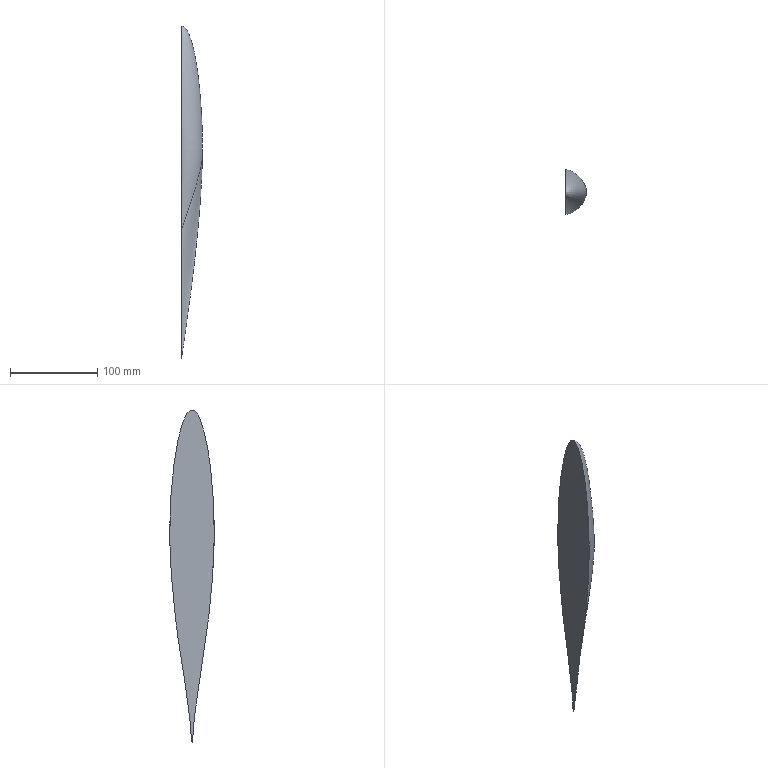Part | SolidWorks | features BaseBody 1 | 1 solid | 3 faces | box 24 x 51.061 x 380.477 mm | volume 163544 mm3 | spline 2 | plane 1